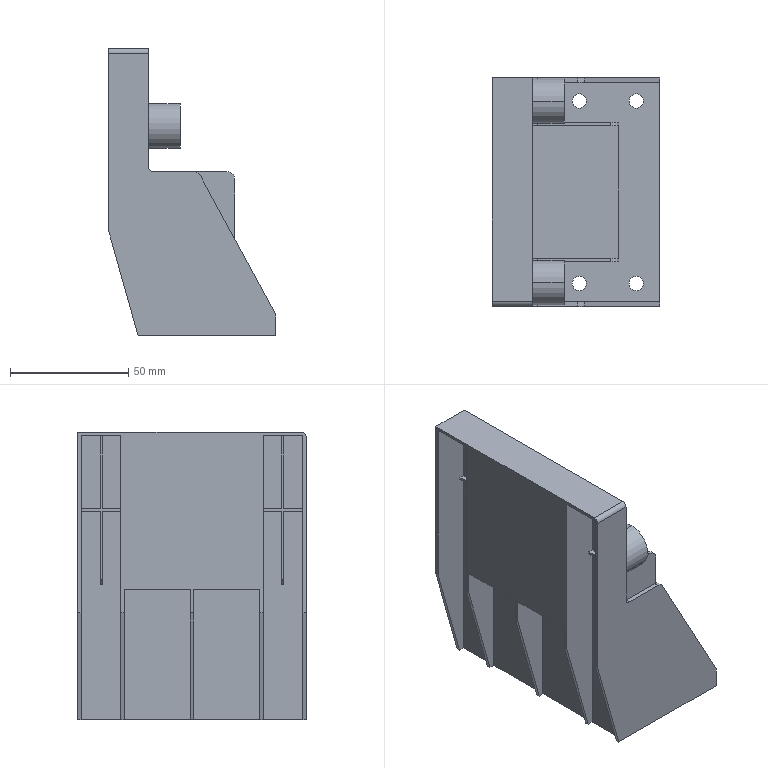Part | NX | features BREP 3 | 3 solids | 139 faces | box 70.8 x 96.5 x 121.2 mm | volume 76427 mm3 | plane 89 | cylinder 42 | cone 8 | commonest cylinder face diameters 12 x12 6 x8 4 x5 6.8 x4 7 x4 10 x4